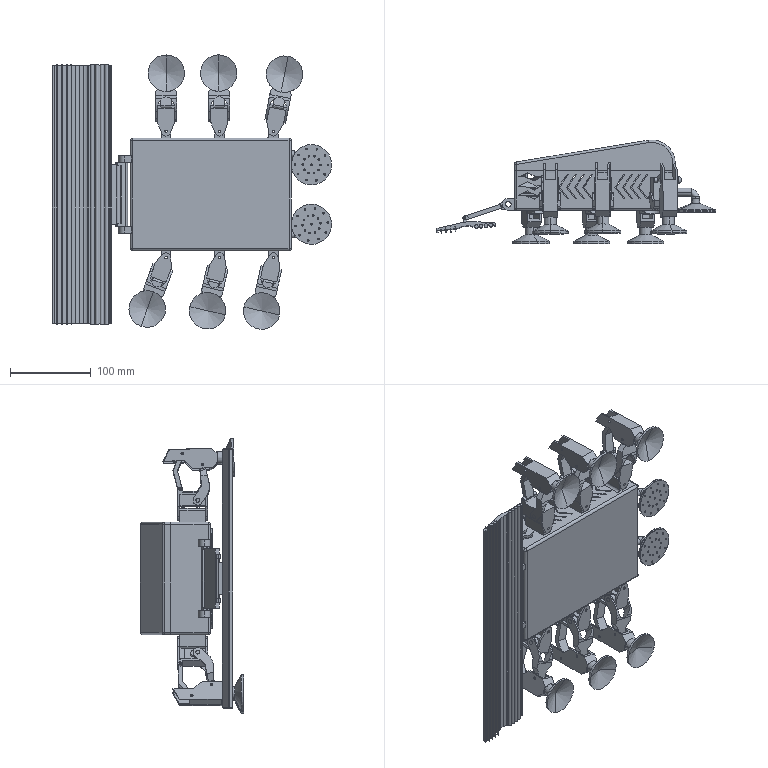Part | SolidWorks | 60 solids | 2608 faces | box 346.952 x 128.874 x 340.963 mm | volume 1244535 mm3 | plane 1520 | cylinder 832 | cone 90 | torus 67 | spline 65 | sphere 34 | commonest cylinder face diameters 3 x185 2 x107 6 x90 5 x66 12 x53 25.162 x40